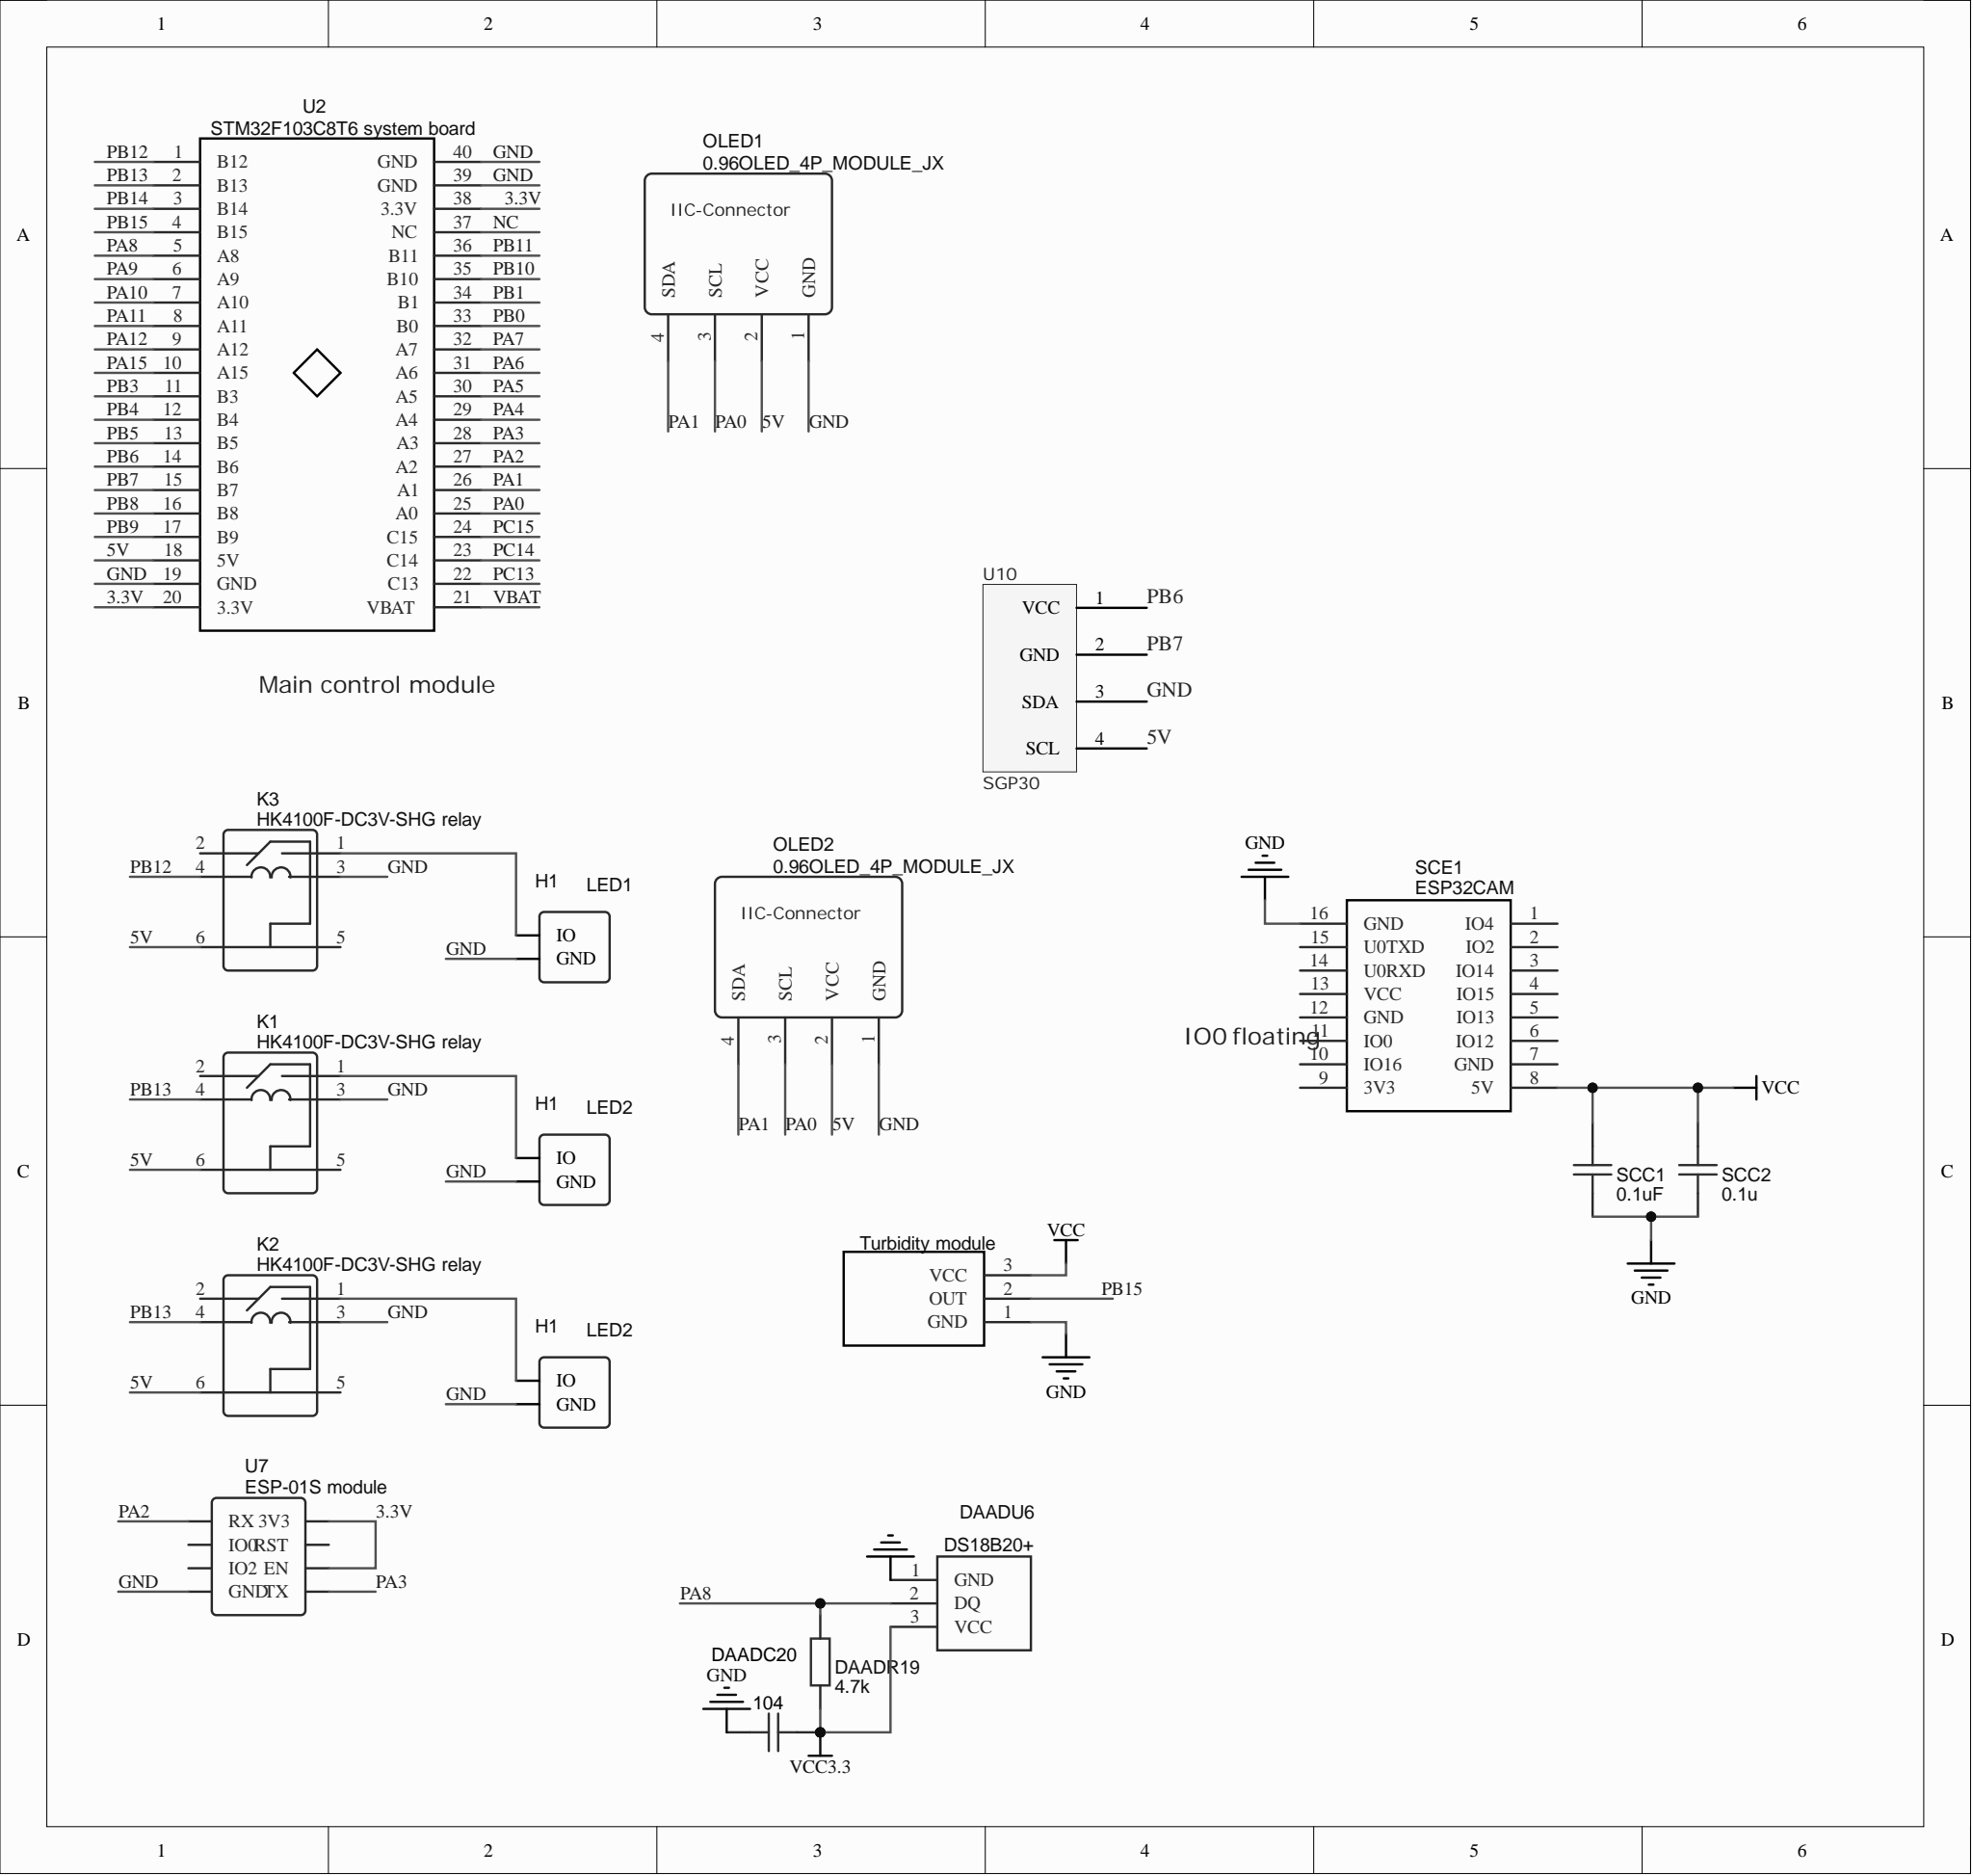Circuit board | Altium Designer | 18 parts | 18 nets
Bill of materials:
Comment,Description,Designator,Footprint,LibRef,Quantity
"104","","DAADC20","C0603","104","1"
"4.7k","","DAADR19","AXIAL-0.3","4.7k","1"
"DS18B20+","","DAADU6","DS18B20","DS18B20+","1"
"HK4100F-DC3V-SHG relay","","K1, K2, K3","HK4100F","HK4100F-DC3V-SHG继电器","3"
"0.96OLED_4P_MODULE_JX","","OLED1, OLED2","0.96OLED_4P","0.96OLED_4P_MODULE_JX","2"
"0.1uF","","SCC1","C0603","0.1uF","1"
"0.1u","","SCC2","C0603","0.1u","1"
"ESP32CAM","","SCE1","ESP32CAM","ESP32CAM","1"
"DC motor terminal","","U1, U3, U5","HDR1X2","直流电机端子","3"
"STM32F103C8T6 system board","","U2","STM32核心板","STM32F103C8T6系统板","1"
"Turbidity module","","U6","HDR1X3","浑浊度模块","1"
"ESP-01S module","","U7","WIFI","ESP-01S模块","1"
"SGP30","","U10","SGP30","SGP30","1"
Netlist (Protel format):
[
DAADC20
C0603
104



]
[
DAADR19
AXIAL-0.3
4.7k



]
[
DAADU6
DS18B20
DS18B20+



]
[
K1
HK4100F
HK4100F-DC3V-SHG relay



]
[
K2
HK4100F
HK4100F-DC3V-SHG relay



]
[
K3
HK4100F
HK4100F-DC3V-SHG relay



]
[
OLED1
0.96OLED_4P
0.96OLED_4P_MODULE_JX



]
[
OLED2
0.96OLED_4P
0.96OLED_4P_MODULE_JX



]
[
SCC1
C0603
0.1uF



]
[
SCC2
C0603
0.1u



]
[
SCE1
ESP32CAM
ESP32CAM



]
[
U1
HDR1X2
DC motor terminal



]
[
U2
STM32核心板
STM32F103C8T6 system board



]
[
U3
HDR1X2
DC motor terminal



]
[
U5
hdr1x2
DC motor terminal



]
[
U6
HDR1X3
Turbidity module



]
[
U7
WIFI
ESP-01S module



]
[
U10
SGP30
SGP30



]
(
VCC3.3
DAADC20-2
DAADR19-1
DAADU6-3
)
(
VCC
SCC1-2
SCC2-2
SCE1-8
U6-3
)
(
PB15
U2-4
U6-2
)
(
PB13
K1-4
K2-4
U2-2
)
(
PB12
K3-4
U2-1
)
(
PB7
U2-15
U10-2
)
(
PB6
U2-14
U10-1
)
(
PA8
DAADR19-2
DAADU6-2
U2-5
)
(
PA3
U2-28
U7-4
)
(
PA2
U2-27
U7-8
)
(
PA1
OLED1-4
OLED2-4
U2-26
)
(
PA0
OLED1-3
OLED2-3
U2-25
)
(
NetK3_1
K3-1
U5-1
)
(
NetK2_1
K2-1
U3-1
)
(
NetK1_1
K1-1
U1-1
)
(
GND
DAADC20-1
DAADU6-1
K1-3
K2-3
K3-3
OLED1-1
OLED2-1
SCC1-1
SCC2-1
SCE1-16
U1-2
U2-19
U2-39
U2-40
U3-2
U5-2
U6-1
U7-5
U10-3
)
(
5V
K1-6
K2-6
K3-6
OLED1-2
OLED2-2
U2-18
U10-4
)
(
3.3V
U2-20
U2-38
U7-1
U7-3
)